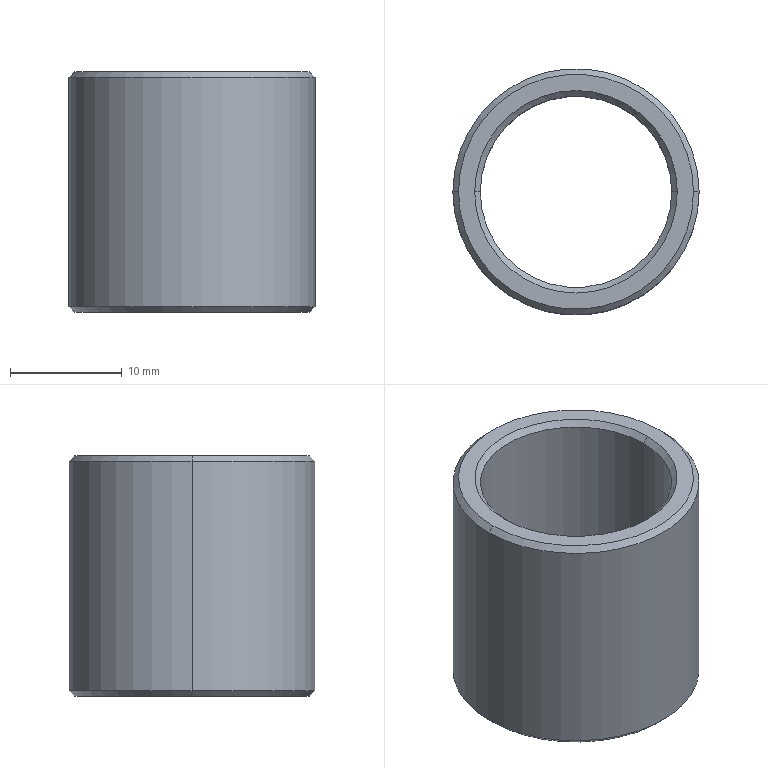Part | SolidWorks | features Chamfer 1, Extrusion 1 | 1 solid | 14 faces | box 22 x 22 x 21.5 mm | volume 3204 mm3 | cone 8 | cylinder 4 | plane 2 | commonest cylinder face diameters 17.1 x2 22 x2
STEP:
#1=CARTESIAN_POINT('',(10.5,0.,21.5));
#2=VERTEX_POINT('',#1);
#3=CARTESIAN_POINT('',(-10.5,0.,21.5));
#4=VERTEX_POINT('',#3);
#5=CARTESIAN_POINT('',(0.,0.,21.5));
#6=DIRECTION('',(0.,0.,1.));
#7=DIRECTION('',(1.,0.,0.));
#8=AXIS2_PLACEMENT_3D('',#5,#6,#7);
#9=CIRCLE('',#8,10.5);
#10=EDGE_CURVE('',#2,#4,#9,.T.);
#11=ORIENTED_EDGE('',*,*,#10,.F.);
#12=CARTESIAN_POINT('',(11.,0.,21.));
#13=VERTEX_POINT('',#12);
#14=CARTESIAN_POINT('',(10.5,0.,21.5));
#15=DIRECTION('',(0.7071,0.,-0.7071));
#16=VECTOR('',#15,1000.);
#17=LINE('',#14,#16);
#18=EDGE_CURVE('',#2,#13,#17,.T.);
#19=ORIENTED_EDGE('',*,*,#18,.T.);
#20=CARTESIAN_POINT('',(-11.,0.,21.));
#21=VERTEX_POINT('',#20);
#22=CARTESIAN_POINT('',(0.,0.,21.));
#23=DIRECTION('',(0.,0.,-1.));
#24=DIRECTION('',(1.,0.,0.));
#25=AXIS2_PLACEMENT_3D('',#22,#23,#24);
#26=CIRCLE('',#25,11.);
#27=EDGE_CURVE('',#21,#13,#26,.T.);
#28=ORIENTED_EDGE('',*,*,#27,.F.);
#29=CARTESIAN_POINT('',(-10.5,0.,21.5));
#30=DIRECTION('',(-0.7071,0.,-0.7071));
#31=VECTOR('',#30,1000.);
#32=LINE('',#29,#31);
#33=EDGE_CURVE('',#4,#21,#32,.T.);
#34=ORIENTED_EDGE('',*,*,#33,.F.);
#35=EDGE_LOOP('',(#11,#19,#28,#34));
#36=FACE_OUTER_BOUND('',#35,.T.);
#37=CARTESIAN_POINT('',(0.,0.,21.5));
#38=DIRECTION('',(0.,0.,-1.));
#39=DIRECTION('',(-1.,0.,0.));
#40=AXIS2_PLACEMENT_3D('',#37,#38,#39);
#41=CONICAL_SURFACE('',#40,10.5,0.7854);
#42=ADVANCED_FACE('',(#36),#41,.T.);
#43=CARTESIAN_POINT('',(-8.55,0.,21.));
#44=VERTEX_POINT('',#43);
#45=CARTESIAN_POINT('',(8.55,0.,21.));
#46=VERTEX_POINT('',#45);
#47=CARTESIAN_POINT('',(0.,0.,21.));
#48=DIRECTION('',(0.,0.,1.));
#49=DIRECTION('',(1.,0.,0.));
#50=AXIS2_PLACEMENT_3D('',#47,#48,#49);
#51=CIRCLE('',#50,8.55);
#52=EDGE_CURVE('',#44,#46,#51,.T.);
#53=ORIENTED_EDGE('',*,*,#52,.F.);
#54=CARTESIAN_POINT('',(-9.05,0.,21.5));
#55=VERTEX_POINT('',#54);
#56=CARTESIAN_POINT('',(-8.55,0.,21.));
#57=DIRECTION('',(-0.7071,0.,0.7071));
#58=VECTOR('',#57,1000.);
#59=LINE('',#56,#58);
#60=EDGE_CURVE('',#44,#55,#59,.T.);
#61=ORIENTED_EDGE('',*,*,#60,.T.);
#62=CARTESIAN_POINT('',(9.05,0.,21.5));
#63=VERTEX_POINT('',#62);
#64=CARTESIAN_POINT('',(0.,0.,21.5));
#65=DIRECTION('',(0.,0.,-1.));
#66=DIRECTION('',(1.,0.,0.));
#67=AXIS2_PLACEMENT_3D('',#64,#65,#66);
#68=CIRCLE('',#67,9.05);
#69=EDGE_CURVE('',#63,#55,#68,.T.);
#70=ORIENTED_EDGE('',*,*,#69,.F.);
#71=CARTESIAN_POINT('',(8.55,0.,21.));
#72=DIRECTION('',(0.7071,0.,0.7071));
#73=VECTOR('',#72,1000.);
#74=LINE('',#71,#73);
#75=EDGE_CURVE('',#46,#63,#74,.T.);
#76=ORIENTED_EDGE('',*,*,#75,.F.);
#77=EDGE_LOOP('',(#53,#61,#70,#76));
#78=FACE_OUTER_BOUND('',#77,.T.);
#79=CARTESIAN_POINT('',(0.,0.,21.));
#80=DIRECTION('',(0.,0.,1.));
#81=DIRECTION('',(1.,0.,0.));
#82=AXIS2_PLACEMENT_3D('',#79,#80,#81);
#83=CONICAL_SURFACE('',#82,8.55,0.7854);
#84=ADVANCED_FACE('',(#78),#83,.F.);
#85=CARTESIAN_POINT('',(-10.5,0.,0.));
#86=VERTEX_POINT('',#85);
#87=CARTESIAN_POINT('',(10.5,0.,0.));
#88=VERTEX_POINT('',#87);
#89=CARTESIAN_POINT('',(0.,0.,0.));
#90=DIRECTION('',(0.,0.,-1.));
#91=DIRECTION('',(1.,0.,0.));
#92=AXIS2_PLACEMENT_3D('',#89,#90,#91);
#93=CIRCLE('',#92,10.5);
#94=EDGE_CURVE('',#86,#88,#93,.T.);
#95=ORIENTED_EDGE('',*,*,#94,.F.);
#96=CARTESIAN_POINT('',(-11.,0.,0.5));
#97=VERTEX_POINT('',#96);
#98=CARTESIAN_POINT('',(-11.,0.,0.5));
#99=DIRECTION('',(-0.7071,0.,0.7071));
#100=VECTOR('',#99,1000.);
#101=LINE('',#98,#100);
#102=EDGE_CURVE('',#86,#97,#101,.T.);
#103=ORIENTED_EDGE('',*,*,#102,.T.);
#104=CARTESIAN_POINT('',(11.,0.,0.5));
#105=VERTEX_POINT('',#104);
#106=CARTESIAN_POINT('',(0.,0.,0.5));
#107=DIRECTION('',(0.,0.,1.));
#108=DIRECTION('',(1.,0.,0.));
#109=AXIS2_PLACEMENT_3D('',#106,#107,#108);
#110=CIRCLE('',#109,11.);
#111=EDGE_CURVE('',#105,#97,#110,.T.);
#112=ORIENTED_EDGE('',*,*,#111,.F.);
#113=CARTESIAN_POINT('',(11.,0.,0.5));
#114=DIRECTION('',(0.7071,0.,0.7071));
#115=VECTOR('',#114,1000.);
#116=LINE('',#113,#115);
#117=EDGE_CURVE('',#88,#105,#116,.T.);
#118=ORIENTED_EDGE('',*,*,#117,.F.);
#119=EDGE_LOOP('',(#95,#103,#112,#118));
#120=FACE_OUTER_BOUND('',#119,.T.);
#121=CARTESIAN_POINT('',(0.,0.,0.5));
#122=DIRECTION('',(0.,0.,1.));
#123=DIRECTION('',(1.,0.,0.));
#124=AXIS2_PLACEMENT_3D('',#121,#122,#123);
#125=CONICAL_SURFACE('',#124,11.,0.7854);
#126=ADVANCED_FACE('',(#120),#125,.T.);
#127=CARTESIAN_POINT('',(8.55,0.,0.5));
#128=VERTEX_POINT('',#127);
#129=CARTESIAN_POINT('',(-8.55,0.,0.5));
#130=VERTEX_POINT('',#129);
#131=CARTESIAN_POINT('',(0.,0.,0.5));
#132=DIRECTION('',(0.,0.,-1.));
#133=DIRECTION('',(1.,0.,0.));
#134=AXIS2_PLACEMENT_3D('',#131,#132,#133);
#135=CIRCLE('',#134,8.55);
#136=EDGE_CURVE('',#128,#130,#135,.T.);
#137=ORIENTED_EDGE('',*,*,#136,.F.);
#138=CARTESIAN_POINT('',(9.05,0.,0.));
#139=VERTEX_POINT('',#138);
#140=CARTESIAN_POINT('',(9.05,0.,0.));
#141=DIRECTION('',(0.7071,0.,-0.7071));
#142=VECTOR('',#141,1000.);
#143=LINE('',#140,#142);
#144=EDGE_CURVE('',#128,#139,#143,.T.);
#145=ORIENTED_EDGE('',*,*,#144,.T.);
#146=CARTESIAN_POINT('',(-9.05,0.,0.));
#147=VERTEX_POINT('',#146);
#148=CARTESIAN_POINT('',(0.,0.,0.));
#149=DIRECTION('',(0.,0.,1.));
#150=DIRECTION('',(1.,0.,0.));
#151=AXIS2_PLACEMENT_3D('',#148,#149,#150);
#152=CIRCLE('',#151,9.05);
#153=EDGE_CURVE('',#147,#139,#152,.T.);
#154=ORIENTED_EDGE('',*,*,#153,.F.);
#155=CARTESIAN_POINT('',(-9.05,0.,0.));
#156=DIRECTION('',(-0.7071,0.,-0.7071));
#157=VECTOR('',#156,1000.);
#158=LINE('',#155,#157);
#159=EDGE_CURVE('',#130,#147,#158,.T.);
#160=ORIENTED_EDGE('',*,*,#159,.F.);
#161=EDGE_LOOP('',(#137,#145,#154,#160));
#162=FACE_OUTER_BOUND('',#161,.T.);
#163=CARTESIAN_POINT('',(0.,0.,0.));
#164=DIRECTION('',(0.,0.,-1.));
#165=DIRECTION('',(-1.,0.,0.));
#166=AXIS2_PLACEMENT_3D('',#163,#164,#165);
#167=CONICAL_SURFACE('',#166,9.05,0.7854);
#168=ADVANCED_FACE('',(#162),#167,.F.);
#169=ORIENTED_EDGE('',*,*,#52,.T.);
#170=CARTESIAN_POINT('',(8.55,0.,21.5));
#171=DIRECTION('',(0.,0.,-1.));
#172=VECTOR('',#171,1000.);
#173=LINE('',#170,#172);
#174=EDGE_CURVE('',#46,#128,#173,.T.);
#175=ORIENTED_EDGE('',*,*,#174,.T.);
#176=ORIENTED_EDGE('',*,*,#136,.T.);
#177=CARTESIAN_POINT('',(-8.55,0.,21.5));
#178=DIRECTION('',(0.,0.,-1.));
#179=VECTOR('',#178,1000.);
#180=LINE('',#177,#179);
#181=EDGE_CURVE('',#44,#130,#180,.T.);
#182=ORIENTED_EDGE('',*,*,#181,.F.);
#183=EDGE_LOOP('',(#169,#175,#176,#182));
#184=FACE_OUTER_BOUND('',#183,.T.);
#185=CARTESIAN_POINT('',(0.,0.,21.5));
#186=DIRECTION('',(0.,0.,-1.));
#187=DIRECTION('',(-1.,0.,0.));
#188=AXIS2_PLACEMENT_3D('',#185,#186,#187);
#189=CYLINDRICAL_SURFACE('',#188,8.55);
#190=ADVANCED_FACE('',(#184),#189,.F.);
#191=ORIENTED_EDGE('',*,*,#27,.T.);
#192=CARTESIAN_POINT('',(11.,0.,21.5));
#193=DIRECTION('',(0.,0.,-1.));
#194=VECTOR('',#193,1000.);
#195=LINE('',#192,#194);
#196=EDGE_CURVE('',#13,#105,#195,.T.);
#197=ORIENTED_EDGE('',*,*,#196,.T.);
#198=ORIENTED_EDGE('',*,*,#111,.T.);
#199=CARTESIAN_POINT('',(-11.,0.,21.5));
#200=DIRECTION('',(0.,0.,-1.));
#201=VECTOR('',#200,1000.);
#202=LINE('',#199,#201);
#203=EDGE_CURVE('',#21,#97,#202,.T.);
#204=ORIENTED_EDGE('',*,*,#203,.F.);
#205=EDGE_LOOP('',(#191,#197,#198,#204));
#206=FACE_OUTER_BOUND('',#205,.T.);
#207=CARTESIAN_POINT('',(0.,0.,21.5));
#208=DIRECTION('',(0.,0.,-1.));
#209=DIRECTION('',(-1.,0.,0.));
#210=AXIS2_PLACEMENT_3D('',#207,#208,#209);
#211=CYLINDRICAL_SURFACE('',#210,11.);
#212=ADVANCED_FACE('',(#206),#211,.T.);
#213=ORIENTED_EDGE('',*,*,#69,.T.);
#214=CARTESIAN_POINT('',(0.,0.,21.5));
#215=DIRECTION('',(0.,0.,-1.));
#216=DIRECTION('',(1.,0.,0.));
#217=AXIS2_PLACEMENT_3D('',#214,#215,#216);
#218=CIRCLE('',#217,9.05);
#219=EDGE_CURVE('',#55,#63,#218,.T.);
#220=ORIENTED_EDGE('',*,*,#219,.T.);
#221=EDGE_LOOP('',(#213,#220));
#222=FACE_BOUND('',#221,.T.);
#223=CARTESIAN_POINT('',(0.,0.,21.5));
#224=DIRECTION('',(0.,0.,1.));
#225=DIRECTION('',(1.,0.,0.));
#226=AXIS2_PLACEMENT_3D('',#223,#224,#225);
#227=CIRCLE('',#226,10.5);
#228=EDGE_CURVE('',#4,#2,#227,.T.);
#229=ORIENTED_EDGE('',*,*,#228,.T.);
#230=ORIENTED_EDGE('',*,*,#10,.T.);
#231=EDGE_LOOP('',(#229,#230));
#232=FACE_OUTER_BOUND('',#231,.T.);
#233=CARTESIAN_POINT('',(0.,0.,21.5));
#234=DIRECTION('',(0.,0.,1.));
#235=DIRECTION('',(1.,0.,0.));
#236=AXIS2_PLACEMENT_3D('',#233,#234,#235);
#237=PLANE('',#236);
#238=ADVANCED_FACE('',(#222,#232),#237,.T.);
#239=ORIENTED_EDGE('',*,*,#153,.T.);
#240=CARTESIAN_POINT('',(0.,0.,0.));
#241=DIRECTION('',(0.,0.,1.));
#242=DIRECTION('',(1.,0.,0.));
#243=AXIS2_PLACEMENT_3D('',#240,#241,#242);
#244=CIRCLE('',#243,9.05);
#245=EDGE_CURVE('',#139,#147,#244,.T.);
#246=ORIENTED_EDGE('',*,*,#245,.T.);
#247=EDGE_LOOP('',(#239,#246));
#248=FACE_BOUND('',#247,.T.);
#249=CARTESIAN_POINT('',(0.,0.,0.));
#250=DIRECTION('',(0.,0.,-1.));
#251=DIRECTION('',(1.,0.,0.));
#252=AXIS2_PLACEMENT_3D('',#249,#250,#251);
#253=CIRCLE('',#252,10.5);
#254=EDGE_CURVE('',#88,#86,#253,.T.);
#255=ORIENTED_EDGE('',*,*,#254,.T.);
#256=ORIENTED_EDGE('',*,*,#94,.T.);
#257=EDGE_LOOP('',(#255,#256));
#258=FACE_OUTER_BOUND('',#257,.T.);
#259=CARTESIAN_POINT('',(0.,0.,0.));
#260=DIRECTION('',(0.,0.,1.));
#261=DIRECTION('',(1.,0.,0.));
#262=AXIS2_PLACEMENT_3D('',#259,#260,#261);
#263=PLANE('',#262);
#264=ADVANCED_FACE('',(#248,#258),#263,.F.);
#265=ORIENTED_EDGE('',*,*,#196,.F.);
#266=CARTESIAN_POINT('',(0.,0.,21.));
#267=DIRECTION('',(0.,0.,-1.));
#268=DIRECTION('',(1.,0.,0.));
#269=AXIS2_PLACEMENT_3D('',#266,#267,#268);
#270=CIRCLE('',#269,11.);
#271=EDGE_CURVE('',#13,#21,#270,.T.);
#272=ORIENTED_EDGE('',*,*,#271,.T.);
#273=ORIENTED_EDGE('',*,*,#203,.T.);
#274=CARTESIAN_POINT('',(0.,0.,0.5));
#275=DIRECTION('',(0.,0.,1.));
#276=DIRECTION('',(1.,0.,0.));
#277=AXIS2_PLACEMENT_3D('',#274,#275,#276);
#278=CIRCLE('',#277,11.);
#279=EDGE_CURVE('',#97,#105,#278,.T.);
#280=ORIENTED_EDGE('',*,*,#279,.T.);
#281=EDGE_LOOP('',(#265,#272,#273,#280));
#282=FACE_OUTER_BOUND('',#281,.T.);
#283=CARTESIAN_POINT('',(0.,0.,21.5));
#284=DIRECTION('',(0.,0.,-1.));
#285=DIRECTION('',(-1.,0.,0.));
#286=AXIS2_PLACEMENT_3D('',#283,#284,#285);
#287=CYLINDRICAL_SURFACE('',#286,11.);
#288=ADVANCED_FACE('',(#282),#287,.T.);
#289=ORIENTED_EDGE('',*,*,#174,.F.);
#290=CARTESIAN_POINT('',(0.,0.,21.));
#291=DIRECTION('',(0.,0.,1.));
#292=DIRECTION('',(1.,0.,0.));
#293=AXIS2_PLACEMENT_3D('',#290,#291,#292);
#294=CIRCLE('',#293,8.55);
#295=EDGE_CURVE('',#46,#44,#294,.T.);
#296=ORIENTED_EDGE('',*,*,#295,.T.);
#297=ORIENTED_EDGE('',*,*,#181,.T.);
#298=CARTESIAN_POINT('',(0.,0.,0.5));
#299=DIRECTION('',(0.,0.,-1.));
#300=DIRECTION('',(1.,0.,0.));
#301=AXIS2_PLACEMENT_3D('',#298,#299,#300);
#302=CIRCLE('',#301,8.55);
#303=EDGE_CURVE('',#130,#128,#302,.T.);
#304=ORIENTED_EDGE('',*,*,#303,.T.);
#305=EDGE_LOOP('',(#289,#296,#297,#304));
#306=FACE_OUTER_BOUND('',#305,.T.);
#307=CARTESIAN_POINT('',(0.,0.,21.5));
#308=DIRECTION('',(0.,0.,-1.));
#309=DIRECTION('',(-1.,0.,0.));
#310=AXIS2_PLACEMENT_3D('',#307,#308,#309);
#311=CYLINDRICAL_SURFACE('',#310,8.55);
#312=ADVANCED_FACE('',(#306),#311,.F.);
#313=ORIENTED_EDGE('',*,*,#144,.F.);
#314=ORIENTED_EDGE('',*,*,#303,.F.);
#315=ORIENTED_EDGE('',*,*,#159,.T.);
#316=ORIENTED_EDGE('',*,*,#245,.F.);
#317=EDGE_LOOP('',(#313,#314,#315,#316));
#318=FACE_OUTER_BOUND('',#317,.T.);
#319=CARTESIAN_POINT('',(0.,0.,0.));
#320=DIRECTION('',(0.,0.,-1.));
#321=DIRECTION('',(-1.,0.,0.));
#322=AXIS2_PLACEMENT_3D('',#319,#320,#321);
#323=CONICAL_SURFACE('',#322,9.05,0.7854);
#324=ADVANCED_FACE('',(#318),#323,.F.);
#325=ORIENTED_EDGE('',*,*,#102,.F.);
#326=ORIENTED_EDGE('',*,*,#254,.F.);
#327=ORIENTED_EDGE('',*,*,#117,.T.);
#328=ORIENTED_EDGE('',*,*,#279,.F.);
#329=EDGE_LOOP('',(#325,#326,#327,#328));
#330=FACE_OUTER_BOUND('',#329,.T.);
#331=CARTESIAN_POINT('',(0.,0.,0.5));
#332=DIRECTION('',(0.,0.,1.));
#333=DIRECTION('',(1.,0.,0.));
#334=AXIS2_PLACEMENT_3D('',#331,#332,#333);
#335=CONICAL_SURFACE('',#334,11.,0.7854);
#336=ADVANCED_FACE('',(#330),#335,.T.);
#337=ORIENTED_EDGE('',*,*,#60,.F.);
#338=ORIENTED_EDGE('',*,*,#295,.F.);
#339=ORIENTED_EDGE('',*,*,#75,.T.);
#340=ORIENTED_EDGE('',*,*,#219,.F.);
#341=EDGE_LOOP('',(#337,#338,#339,#340));
#342=FACE_OUTER_BOUND('',#341,.T.);
#343=CARTESIAN_POINT('',(0.,0.,21.));
#344=DIRECTION('',(0.,0.,1.));
#345=DIRECTION('',(1.,0.,0.));
#346=AXIS2_PLACEMENT_3D('',#343,#344,#345);
#347=CONICAL_SURFACE('',#346,8.55,0.7854);
#348=ADVANCED_FACE('',(#342),#347,.F.);
#349=ORIENTED_EDGE('',*,*,#18,.F.);
#350=ORIENTED_EDGE('',*,*,#228,.F.);
#351=ORIENTED_EDGE('',*,*,#33,.T.);
#352=ORIENTED_EDGE('',*,*,#271,.F.);
#353=EDGE_LOOP('',(#349,#350,#351,#352));
#354=FACE_OUTER_BOUND('',#353,.T.);
#355=CARTESIAN_POINT('',(0.,0.,21.5));
#356=DIRECTION('',(0.,0.,-1.));
#357=DIRECTION('',(-1.,0.,0.));
#358=AXIS2_PLACEMENT_3D('',#355,#356,#357);
#359=CONICAL_SURFACE('',#358,10.5,0.7854);
#360=ADVANCED_FACE('',(#354),#359,.T.);
#361=CLOSED_SHELL('',(#42,#84,#126,#168,#190,#212,#238,#264,#288,#312,#324,#336,#348,#360));
#362=MANIFOLD_SOLID_BREP('',#361);
#363=CARTESIAN_POINT('',(0.,0.,0.));
#364=DIRECTION('',(0.,0.,1.));
#365=DIRECTION('',(1.,0.,0.));
#366=AXIS2_PLACEMENT_3D('',#363,#364,#365);
#367=(LENGTH_UNIT()NAMED_UNIT(*)SI_UNIT(.MILLI.,.METRE.));
#368=UNCERTAINTY_MEASURE_WITH_UNIT(LENGTH_MEASURE(0.00001),#367,'','');
#369=(NAMED_UNIT(*)PLANE_ANGLE_UNIT()SI_UNIT($,.RADIAN.));
#370=(NAMED_UNIT(*)SI_UNIT($,.STERADIAN.)SOLID_ANGLE_UNIT());
#371=(GEOMETRIC_REPRESENTATION_CONTEXT(3)GLOBAL_UNCERTAINTY_ASSIGNED_CONTEXT((#368))GLOBAL_UNIT_ASSIGNED_CONTEXT((#367,#369,#370))REPRESENTATION_CONTEXT('',''));
#372=ADVANCED_BREP_SHAPE_REPRESENTATION('',(#362,#366),#371);